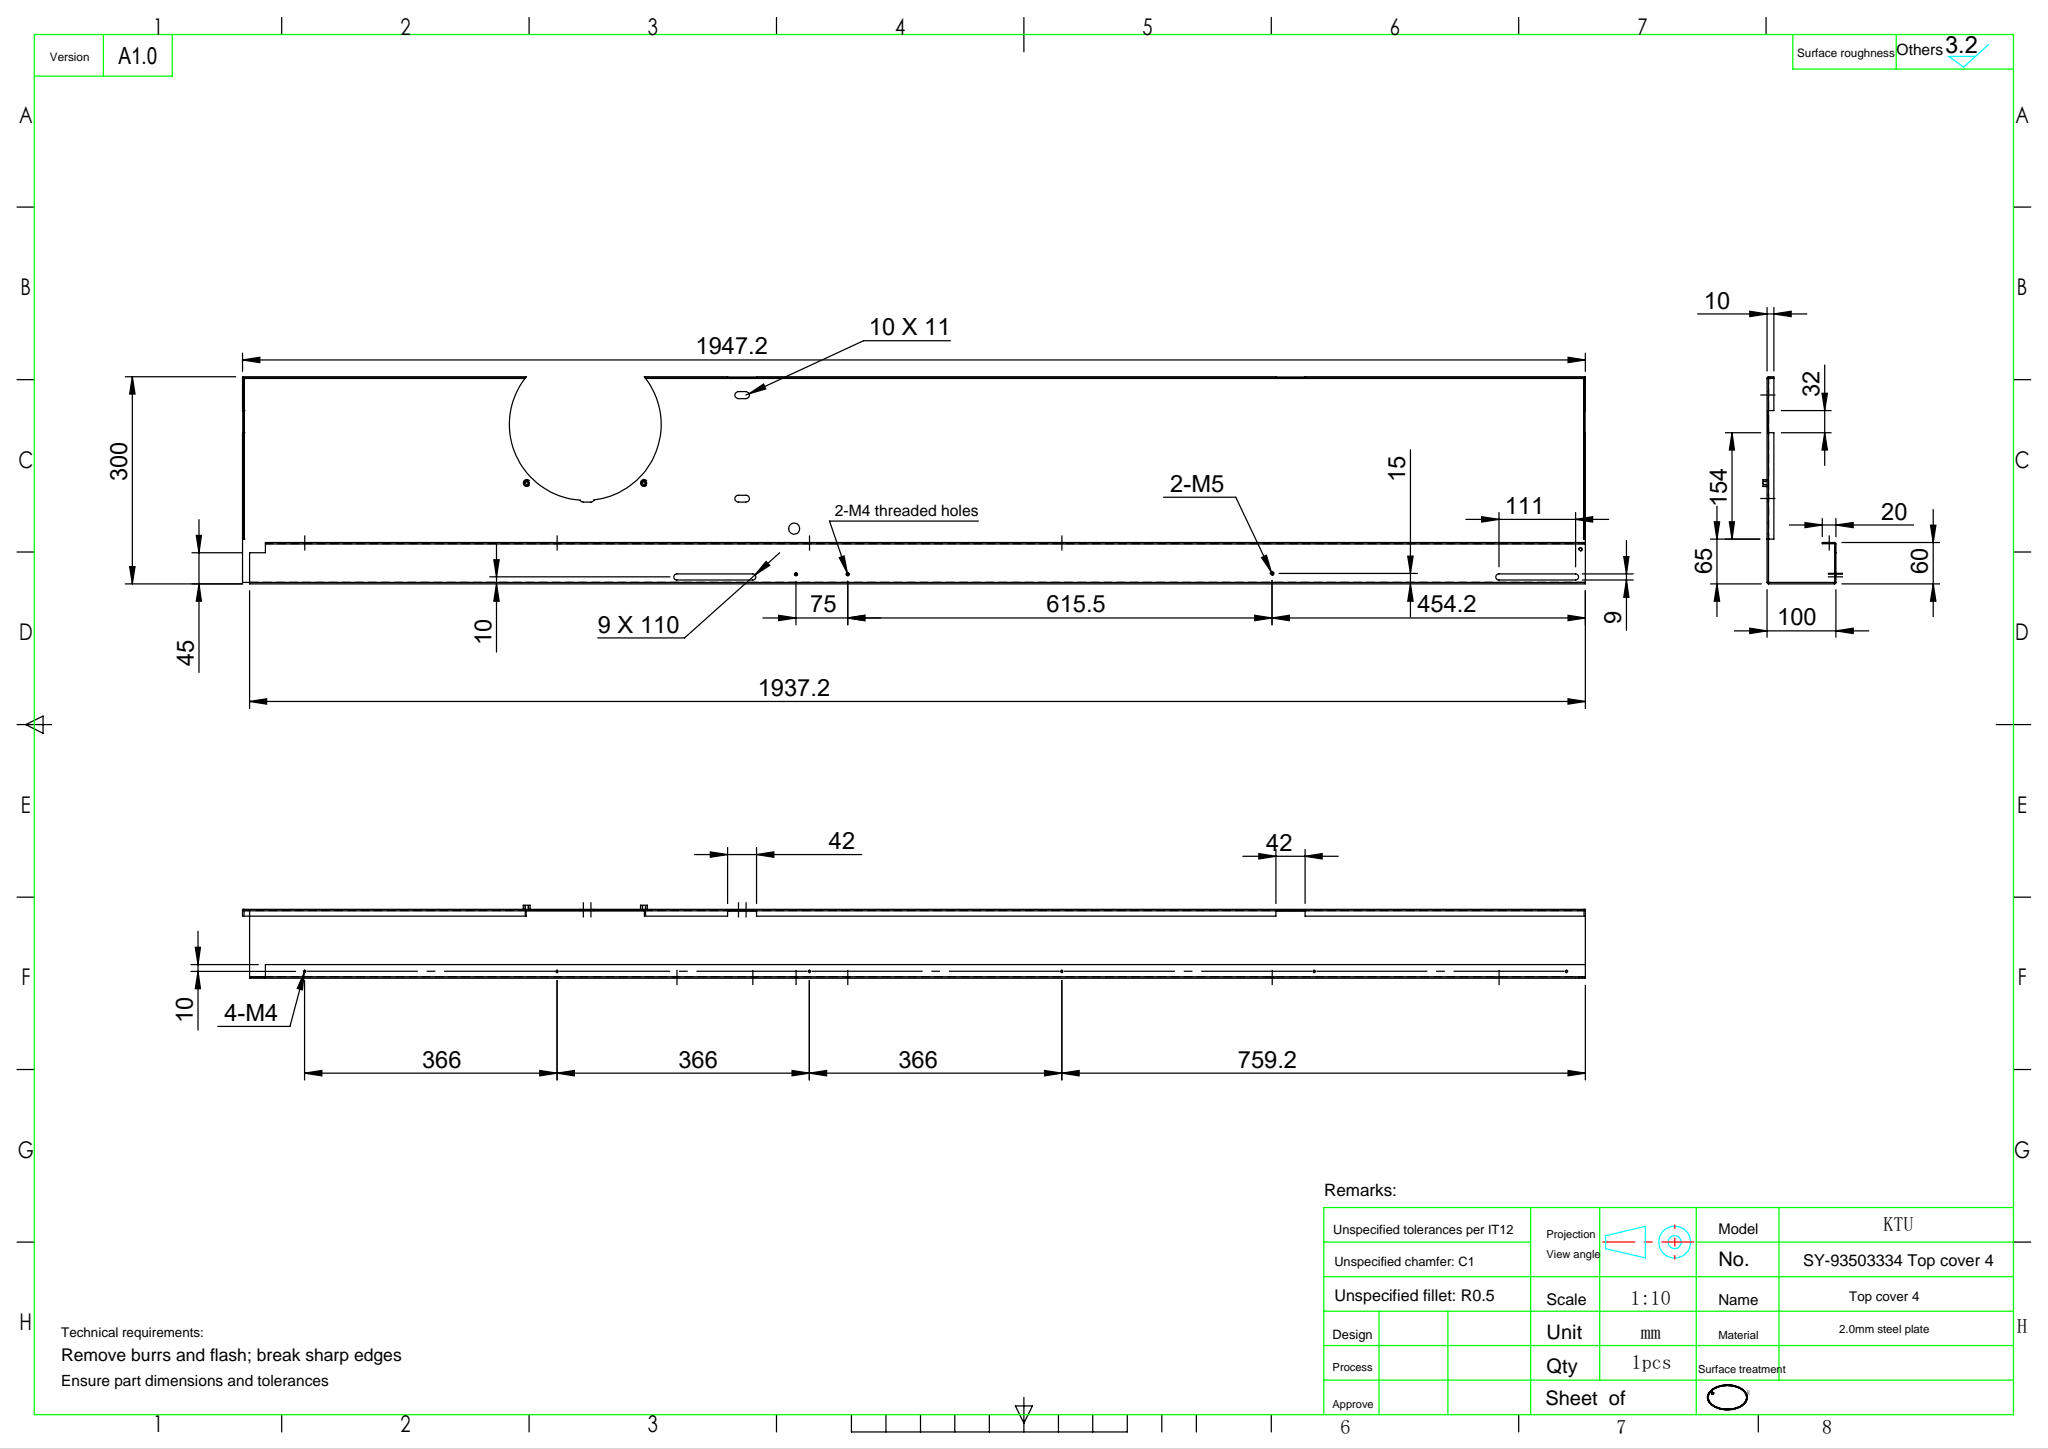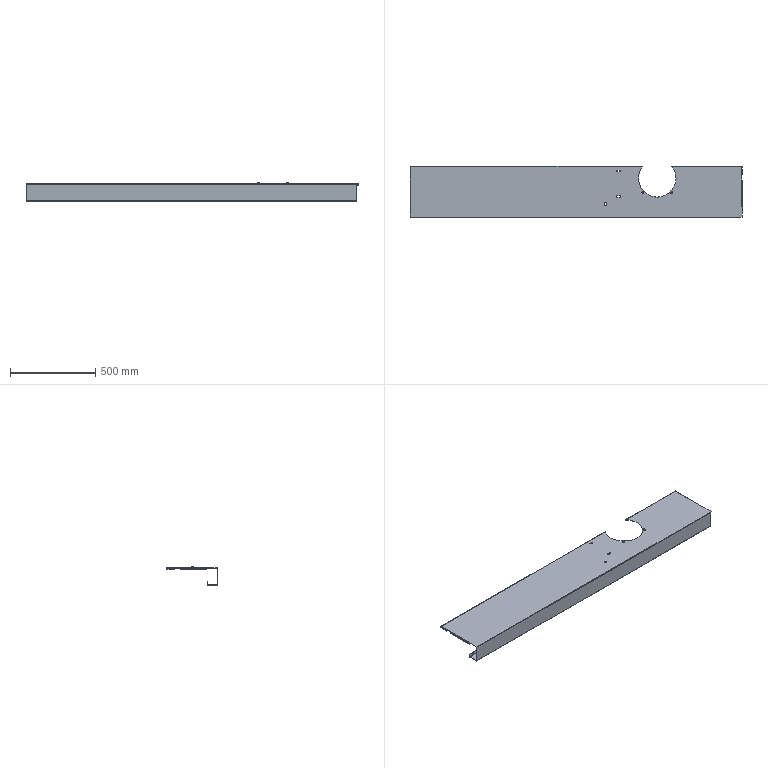Part | SolidWorks | features Cut 7, EdgeFlange 5, HoleWzd 4, ICE 4, LPattern 2, 3DProfileFeature 1, FlatPattern 1, MirrorPattern 1, SMBaseFlange 1, SheetMetal 1 | 1 solid | 166 faces | box 1947 x 300 x 106 mm | volume 1794702 mm3 | plane 97 | cylinder 65 | cone 4 | commonest cylinder face diameters 3.3 x16 10 x12 4.2 x8 0.4 x7 4.4 x7 9 x6